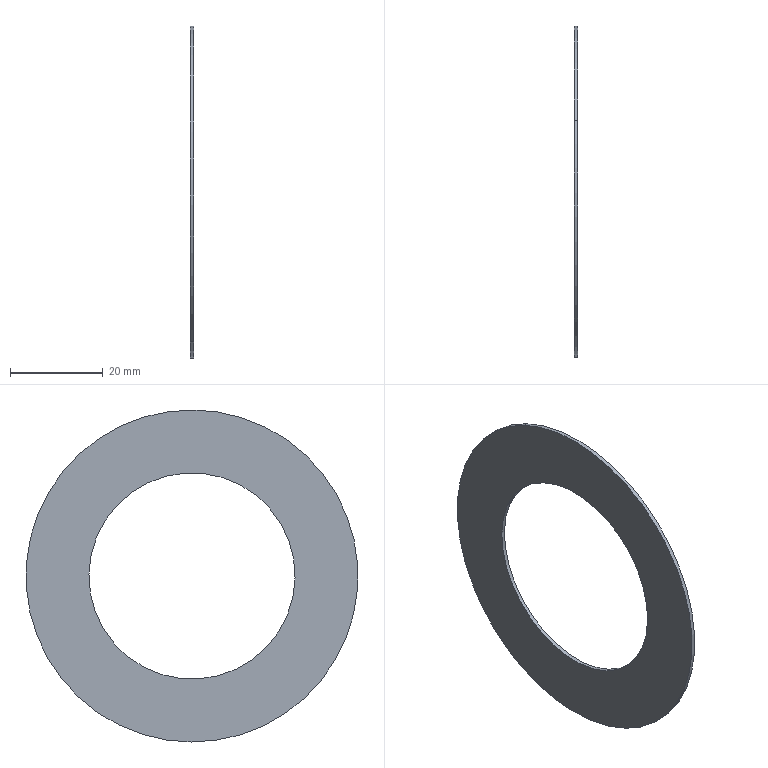Part | NX | features BREP 1 | 1 solid | 6 faces | box 0.8 x 71.5 x 71.5 mm | volume 1973 mm3 | cylinder 4 | plane 2 | commonest cylinder face diameters 44.4 x2 71.5 x2
STEP:
#1=CARTESIAN_POINT('',(70.65,15.336,32.294));
#2=VERTEX_POINT('',#1);
#3=CARTESIAN_POINT('',(70.65,-15.336,-32.294));
#4=VERTEX_POINT('',#3);
#5=CARTESIAN_POINT('',(70.65,0.,0.));
#6=DIRECTION('',(-1.,0.,0.));
#7=DIRECTION('',(0.,0.429,0.9033));
#8=AXIS2_PLACEMENT_3D('',#5,#6,#7);
#9=CIRCLE('',#8,35.75);
#10=EDGE_CURVE('',#2,#4,#9,.T.);
#11=ORIENTED_EDGE('',*,*,#10,.T.);
#12=CARTESIAN_POINT('',(69.85,-15.336,-32.294));
#13=VERTEX_POINT('',#12);
#14=CARTESIAN_POINT('',(69.85,-15.336,-32.294));
#15=DIRECTION('',(-1.,0.,0.));
#16=VECTOR('',#15,1000.);
#17=LINE('',#14,#16);
#18=EDGE_CURVE('',#4,#13,#17,.T.);
#19=ORIENTED_EDGE('',*,*,#18,.T.);
#20=CARTESIAN_POINT('',(69.85,15.336,32.294));
#21=VERTEX_POINT('',#20);
#22=CARTESIAN_POINT('',(69.85,0.,0.));
#23=DIRECTION('',(-1.,0.,0.));
#24=DIRECTION('',(0.,0.429,0.9033));
#25=AXIS2_PLACEMENT_3D('',#22,#23,#24);
#26=CIRCLE('',#25,35.75);
#27=EDGE_CURVE('',#21,#13,#26,.T.);
#28=ORIENTED_EDGE('',*,*,#27,.F.);
#29=CARTESIAN_POINT('',(69.85,15.336,32.294));
#30=DIRECTION('',(-1.,0.,0.));
#31=VECTOR('',#30,1000.);
#32=LINE('',#29,#31);
#33=EDGE_CURVE('',#2,#21,#32,.T.);
#34=ORIENTED_EDGE('',*,*,#33,.F.);
#35=EDGE_LOOP('',(#11,#19,#28,#34));
#36=FACE_BOUND('',#35,.T.);
#37=CARTESIAN_POINT('',(69.85,0.,0.));
#38=DIRECTION('',(-1.,0.,0.));
#39=DIRECTION('',(0.,-0.429,-0.9033));
#40=AXIS2_PLACEMENT_3D('',#37,#38,#39);
#41=CYLINDRICAL_SURFACE('',#40,35.75);
#42=ADVANCED_FACE('',(#36),#41,.T.);
#43=CARTESIAN_POINT('',(70.65,-9.523,-20.054));
#44=VERTEX_POINT('',#43);
#45=CARTESIAN_POINT('',(70.65,9.523,20.054));
#46=VERTEX_POINT('',#45);
#47=CARTESIAN_POINT('',(70.65,0.,0.));
#48=DIRECTION('',(-1.,0.,0.));
#49=DIRECTION('',(0.,0.429,0.9033));
#50=AXIS2_PLACEMENT_3D('',#47,#48,#49);
#51=CIRCLE('',#50,22.2);
#52=EDGE_CURVE('',#44,#46,#51,.T.);
#53=ORIENTED_EDGE('',*,*,#52,.F.);
#54=CARTESIAN_POINT('',(69.85,-9.523,-20.054));
#55=VERTEX_POINT('',#54);
#56=CARTESIAN_POINT('',(69.85,-9.523,-20.054));
#57=DIRECTION('',(-1.,0.,0.));
#58=VECTOR('',#57,1000.);
#59=LINE('',#56,#58);
#60=EDGE_CURVE('',#44,#55,#59,.T.);
#61=ORIENTED_EDGE('',*,*,#60,.T.);
#62=CARTESIAN_POINT('',(69.85,9.523,20.054));
#63=VERTEX_POINT('',#62);
#64=CARTESIAN_POINT('',(69.85,0.,0.));
#65=DIRECTION('',(-1.,0.,0.));
#66=DIRECTION('',(0.,0.429,0.9033));
#67=AXIS2_PLACEMENT_3D('',#64,#65,#66);
#68=CIRCLE('',#67,22.2);
#69=EDGE_CURVE('',#55,#63,#68,.T.);
#70=ORIENTED_EDGE('',*,*,#69,.T.);
#71=CARTESIAN_POINT('',(69.85,9.523,20.054));
#72=DIRECTION('',(-1.,0.,0.));
#73=VECTOR('',#72,1000.);
#74=LINE('',#71,#73);
#75=EDGE_CURVE('',#46,#63,#74,.T.);
#76=ORIENTED_EDGE('',*,*,#75,.F.);
#77=EDGE_LOOP('',(#53,#61,#70,#76));
#78=FACE_BOUND('',#77,.T.);
#79=CARTESIAN_POINT('',(69.85,0.,0.));
#80=DIRECTION('',(-1.,0.,0.));
#81=DIRECTION('',(0.,-0.429,-0.9033));
#82=AXIS2_PLACEMENT_3D('',#79,#80,#81);
#83=CYLINDRICAL_SURFACE('',#82,22.2);
#84=ADVANCED_FACE('',(#78),#83,.F.);
#85=CARTESIAN_POINT('',(69.85,0.,0.));
#86=DIRECTION('',(-1.,0.,0.));
#87=DIRECTION('',(0.,0.429,0.9033));
#88=AXIS2_PLACEMENT_3D('',#85,#86,#87);
#89=CIRCLE('',#88,22.2);
#90=EDGE_CURVE('',#63,#55,#89,.T.);
#91=ORIENTED_EDGE('',*,*,#90,.F.);
#92=ORIENTED_EDGE('',*,*,#69,.F.);
#93=EDGE_LOOP('',(#91,#92));
#94=FACE_BOUND('',#93,.T.);
#95=ORIENTED_EDGE('',*,*,#27,.T.);
#96=CARTESIAN_POINT('',(69.85,0.,0.));
#97=DIRECTION('',(-1.,0.,0.));
#98=DIRECTION('',(0.,0.429,0.9033));
#99=AXIS2_PLACEMENT_3D('',#96,#97,#98);
#100=CIRCLE('',#99,35.75);
#101=EDGE_CURVE('',#13,#21,#100,.T.);
#102=ORIENTED_EDGE('',*,*,#101,.T.);
#103=EDGE_LOOP('',(#95,#102));
#104=FACE_BOUND('',#103,.T.);
#105=CARTESIAN_POINT('',(69.85,32.294,-15.336));
#106=DIRECTION('',(1.,0.,0.));
#107=DIRECTION('',(0.,0.429,0.9033));
#108=AXIS2_PLACEMENT_3D('',#105,#106,#107);
#109=PLANE('',#108);
#110=ADVANCED_FACE('',(#94,#104),#109,.F.);
#111=ORIENTED_EDGE('',*,*,#60,.F.);
#112=CARTESIAN_POINT('',(70.65,0.,0.));
#113=DIRECTION('',(-1.,0.,0.));
#114=DIRECTION('',(0.,0.429,0.9033));
#115=AXIS2_PLACEMENT_3D('',#112,#113,#114);
#116=CIRCLE('',#115,22.2);
#117=EDGE_CURVE('',#46,#44,#116,.T.);
#118=ORIENTED_EDGE('',*,*,#117,.F.);
#119=ORIENTED_EDGE('',*,*,#75,.T.);
#120=ORIENTED_EDGE('',*,*,#90,.T.);
#121=EDGE_LOOP('',(#111,#118,#119,#120));
#122=FACE_BOUND('',#121,.T.);
#123=CARTESIAN_POINT('',(69.85,0.,0.));
#124=DIRECTION('',(-1.,0.,0.));
#125=DIRECTION('',(0.,-0.429,-0.9033));
#126=AXIS2_PLACEMENT_3D('',#123,#124,#125);
#127=CYLINDRICAL_SURFACE('',#126,22.2);
#128=ADVANCED_FACE('',(#122),#127,.F.);
#129=ORIENTED_EDGE('',*,*,#10,.F.);
#130=CARTESIAN_POINT('',(70.65,0.,0.));
#131=DIRECTION('',(-1.,0.,0.));
#132=DIRECTION('',(0.,0.429,0.9033));
#133=AXIS2_PLACEMENT_3D('',#130,#131,#132);
#134=CIRCLE('',#133,35.75);
#135=EDGE_CURVE('',#4,#2,#134,.T.);
#136=ORIENTED_EDGE('',*,*,#135,.F.);
#137=EDGE_LOOP('',(#129,#136));
#138=FACE_BOUND('',#137,.T.);
#139=ORIENTED_EDGE('',*,*,#117,.T.);
#140=ORIENTED_EDGE('',*,*,#52,.T.);
#141=EDGE_LOOP('',(#139,#140));
#142=FACE_BOUND('',#141,.T.);
#143=CARTESIAN_POINT('',(70.65,20.054,-9.523));
#144=DIRECTION('',(-1.,0.,0.));
#145=DIRECTION('',(0.,-0.429,-0.9033));
#146=AXIS2_PLACEMENT_3D('',#143,#144,#145);
#147=PLANE('',#146);
#148=ADVANCED_FACE('',(#138,#142),#147,.F.);
#149=ORIENTED_EDGE('',*,*,#18,.F.);
#150=ORIENTED_EDGE('',*,*,#135,.T.);
#151=ORIENTED_EDGE('',*,*,#33,.T.);
#152=ORIENTED_EDGE('',*,*,#101,.F.);
#153=EDGE_LOOP('',(#149,#150,#151,#152));
#154=FACE_BOUND('',#153,.T.);
#155=CARTESIAN_POINT('',(69.85,0.,0.));
#156=DIRECTION('',(-1.,0.,0.));
#157=DIRECTION('',(0.,-0.429,-0.9033));
#158=AXIS2_PLACEMENT_3D('',#155,#156,#157);
#159=CYLINDRICAL_SURFACE('',#158,35.75);
#160=ADVANCED_FACE('',(#154),#159,.T.);
#161=CLOSED_SHELL('',(#42,#84,#110,#128,#148,#160));
#162=MANIFOLD_SOLID_BREP('',#161);
#163=(LENGTH_UNIT()NAMED_UNIT(*)SI_UNIT(.MILLI.,.METRE.));
#164=UNCERTAINTY_MEASURE_WITH_UNIT(LENGTH_MEASURE(0.00001),#163,'','');
#165=(NAMED_UNIT(*)PLANE_ANGLE_UNIT()SI_UNIT($,.RADIAN.));
#166=(NAMED_UNIT(*)SI_UNIT($,.STERADIAN.)SOLID_ANGLE_UNIT());
#167=(GEOMETRIC_REPRESENTATION_CONTEXT(3)GLOBAL_UNCERTAINTY_ASSIGNED_CONTEXT((#164))GLOBAL_UNIT_ASSIGNED_CONTEXT((#163,#165,#166))REPRESENTATION_CONTEXT('',''));
#168=ADVANCED_BREP_SHAPE_REPRESENTATION('',(#162),#167);